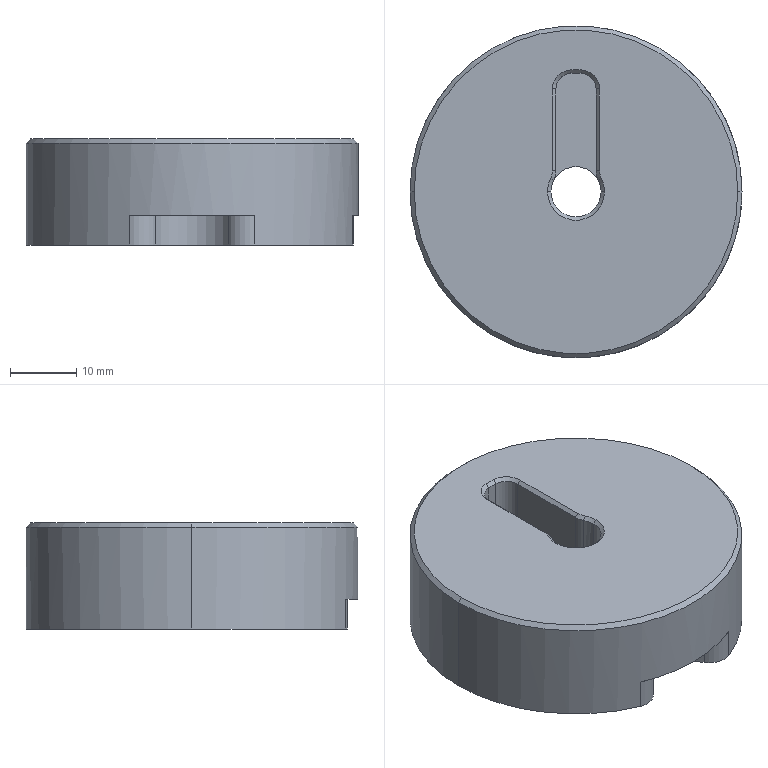Part | 1 solid | 47 faces | box 50.292 x 50.292 x 16.057 mm | volume 28762 mm3 | cylinder 23 | plane 14 | cone 10 | commonest cylinder face diameters 6.35 x8 4.763 x5 5.067 x4 7.62 x2 50.292 x2 12.7 x1
STEP:
#1=CARTESIAN_POINT('',(24.432,-5.556,-16.057));
#2=VERTEX_POINT('',#1);
#3=CARTESIAN_POINT('',(24.329,-6.359,-16.057));
#4=VERTEX_POINT('',#3);
#5=CARTESIAN_POINT('',(21.257,-5.556,-16.057));
#6=DIRECTION('',(0.,0.,-1.));
#7=DIRECTION('',(-1.,0.,0.));
#8=AXIS2_PLACEMENT_3D('',#5,#6,#7);
#9=CIRCLE('',#8,3.175);
#10=EDGE_CURVE('',#2,#4,#9,.T.);
#11=ORIENTED_EDGE('',*,*,#10,.F.);
#12=CARTESIAN_POINT('',(24.432,-5.556,-11.579));
#13=VERTEX_POINT('',#12);
#14=CARTESIAN_POINT('',(24.432,-5.556,0.));
#15=DIRECTION('',(0.,0.,-1.));
#16=VECTOR('',#15,1000.);
#17=LINE('',#14,#16);
#18=EDGE_CURVE('',#13,#2,#17,.T.);
#19=ORIENTED_EDGE('',*,*,#18,.F.);
#20=CARTESIAN_POINT('',(24.329,-6.359,-11.579));
#21=VERTEX_POINT('',#20);
#22=CARTESIAN_POINT('',(21.257,-5.556,-11.579));
#23=DIRECTION('',(0.,0.,1.));
#24=DIRECTION('',(1.,0.,0.));
#25=AXIS2_PLACEMENT_3D('',#22,#23,#24);
#26=CIRCLE('',#25,3.175);
#27=EDGE_CURVE('',#21,#13,#26,.T.);
#28=ORIENTED_EDGE('',*,*,#27,.F.);
#29=CARTESIAN_POINT('',(24.329,-6.359,0.));
#30=DIRECTION('',(0.,0.,1.));
#31=VECTOR('',#30,1000.);
#32=LINE('',#29,#31);
#33=EDGE_CURVE('',#4,#21,#32,.T.);
#34=ORIENTED_EDGE('',*,*,#33,.F.);
#35=EDGE_LOOP('',(#11,#19,#28,#34));
#36=FACE_BOUND('',#35,.T.);
#37=CARTESIAN_POINT('',(21.257,-5.556,0.));
#38=DIRECTION('',(0.,0.,-1.));
#39=DIRECTION('',(-1.,0.,0.));
#40=AXIS2_PLACEMENT_3D('',#37,#38,#39);
#41=CYLINDRICAL_SURFACE('',#40,3.175);
#42=ADVANCED_FACE('',(#36),#41,.T.);
#43=CARTESIAN_POINT('',(21.257,-2.381,-16.057));
#44=VERTEX_POINT('',#43);
#45=CARTESIAN_POINT('',(21.257,-5.556,-16.057));
#46=DIRECTION('',(0.,0.,-1.));
#47=DIRECTION('',(-1.,0.,0.));
#48=AXIS2_PLACEMENT_3D('',#45,#46,#47);
#49=CIRCLE('',#48,3.175);
#50=EDGE_CURVE('',#44,#2,#49,.T.);
#51=ORIENTED_EDGE('',*,*,#50,.F.);
#52=CARTESIAN_POINT('',(21.257,-2.381,-11.579));
#53=VERTEX_POINT('',#52);
#54=CARTESIAN_POINT('',(21.257,-2.381,-11.579));
#55=DIRECTION('',(0.,0.,-1.));
#56=VECTOR('',#55,1000.);
#57=LINE('',#54,#56);
#58=EDGE_CURVE('',#53,#44,#57,.T.);
#59=ORIENTED_EDGE('',*,*,#58,.F.);
#60=CARTESIAN_POINT('',(21.257,-5.556,-11.579));
#61=DIRECTION('',(0.,0.,1.));
#62=DIRECTION('',(1.,0.,0.));
#63=AXIS2_PLACEMENT_3D('',#60,#61,#62);
#64=CIRCLE('',#63,3.175);
#65=EDGE_CURVE('',#13,#53,#64,.T.);
#66=ORIENTED_EDGE('',*,*,#65,.F.);
#67=ORIENTED_EDGE('',*,*,#18,.T.);
#68=EDGE_LOOP('',(#51,#59,#66,#67));
#69=FACE_BOUND('',#68,.T.);
#70=CARTESIAN_POINT('',(21.257,-5.556,0.));
#71=DIRECTION('',(0.,0.,-1.));
#72=DIRECTION('',(-1.,0.,0.));
#73=AXIS2_PLACEMENT_3D('',#70,#71,#72);
#74=CYLINDRICAL_SURFACE('',#73,3.175);
#75=ADVANCED_FACE('',(#69),#74,.T.);
#76=ORIENTED_EDGE('',*,*,#58,.T.);
#77=CARTESIAN_POINT('',(12.898,-2.381,-16.057));
#78=VERTEX_POINT('',#77);
#79=CARTESIAN_POINT('',(12.898,-2.381,-16.057));
#80=DIRECTION('',(-1.,0.,0.));
#81=VECTOR('',#80,1000.);
#82=LINE('',#79,#81);
#83=EDGE_CURVE('',#44,#78,#82,.T.);
#84=ORIENTED_EDGE('',*,*,#83,.T.);
#85=CARTESIAN_POINT('',(12.898,-2.381,-11.579));
#86=VERTEX_POINT('',#85);
#87=CARTESIAN_POINT('',(12.898,-2.381,-11.579));
#88=DIRECTION('',(0.,0.,-1.));
#89=VECTOR('',#88,1000.);
#90=LINE('',#87,#89);
#91=EDGE_CURVE('',#86,#78,#90,.T.);
#92=ORIENTED_EDGE('',*,*,#91,.F.);
#93=CARTESIAN_POINT('',(12.898,-2.381,-11.579));
#94=DIRECTION('',(-1.,0.,0.));
#95=VECTOR('',#94,1000.);
#96=LINE('',#93,#95);
#97=EDGE_CURVE('',#53,#86,#96,.T.);
#98=ORIENTED_EDGE('',*,*,#97,.F.);
#99=EDGE_LOOP('',(#76,#84,#92,#98));
#100=FACE_BOUND('',#99,.T.);
#101=CARTESIAN_POINT('',(12.898,-2.381,-11.579));
#102=DIRECTION('',(0.,-1.,0.));
#103=DIRECTION('',(1.,0.,0.));
#104=AXIS2_PLACEMENT_3D('',#101,#102,#103);
#105=PLANE('',#104);
#106=ADVANCED_FACE('',(#100),#105,.F.);
#107=ORIENTED_EDGE('',*,*,#91,.T.);
#108=CARTESIAN_POINT('',(11.168,1.636,-16.057));
#109=VERTEX_POINT('',#108);
#110=CARTESIAN_POINT('',(12.898,0.,-16.057));
#111=DIRECTION('',(0.,0.,-1.));
#112=DIRECTION('',(-1.,0.,0.));
#113=AXIS2_PLACEMENT_3D('',#110,#111,#112);
#114=CIRCLE('',#113,2.381);
#115=EDGE_CURVE('',#78,#109,#114,.T.);
#116=ORIENTED_EDGE('',*,*,#115,.T.);
#117=CARTESIAN_POINT('',(11.168,1.636,-11.579));
#118=VERTEX_POINT('',#117);
#119=CARTESIAN_POINT('',(11.168,1.636,-11.579));
#120=DIRECTION('',(0.,0.,-1.));
#121=VECTOR('',#120,1000.);
#122=LINE('',#119,#121);
#123=EDGE_CURVE('',#118,#109,#122,.T.);
#124=ORIENTED_EDGE('',*,*,#123,.F.);
#125=CARTESIAN_POINT('',(12.898,0.,-11.579));
#126=DIRECTION('',(0.,0.,-1.));
#127=DIRECTION('',(1.,0.,0.));
#128=AXIS2_PLACEMENT_3D('',#125,#126,#127);
#129=CIRCLE('',#128,2.381);
#130=EDGE_CURVE('',#86,#118,#129,.T.);
#131=ORIENTED_EDGE('',*,*,#130,.F.);
#132=EDGE_LOOP('',(#107,#116,#124,#131));
#133=FACE_BOUND('',#132,.T.);
#134=CARTESIAN_POINT('',(12.898,0.,-11.579));
#135=DIRECTION('',(0.,0.,-1.));
#136=DIRECTION('',(-1.,0.,0.));
#137=AXIS2_PLACEMENT_3D('',#134,#135,#136);
#138=CYLINDRICAL_SURFACE('',#137,2.381);
#139=ADVANCED_FACE('',(#133),#138,.F.);
#140=ORIENTED_EDGE('',*,*,#123,.T.);
#141=CARTESIAN_POINT('',(19.946,10.918,-16.057));
#142=VERTEX_POINT('',#141);
#143=CARTESIAN_POINT('',(16.338,7.102,-16.057));
#144=DIRECTION('',(0.6871,0.7266,0.));
#145=VECTOR('',#144,1000.);
#146=LINE('',#143,#145);
#147=EDGE_CURVE('',#109,#142,#146,.T.);
#148=ORIENTED_EDGE('',*,*,#147,.T.);
#149=CARTESIAN_POINT('',(19.946,10.918,-11.579));
#150=VERTEX_POINT('',#149);
#151=CARTESIAN_POINT('',(19.946,10.918,-11.579));
#152=DIRECTION('',(0.,0.,1.));
#153=VECTOR('',#152,1000.);
#154=LINE('',#151,#153);
#155=EDGE_CURVE('',#142,#150,#154,.T.);
#156=ORIENTED_EDGE('',*,*,#155,.T.);
#157=CARTESIAN_POINT('',(16.338,7.102,-11.579));
#158=DIRECTION('',(0.6871,0.7266,0.));
#159=VECTOR('',#158,1000.);
#160=LINE('',#157,#159);
#161=EDGE_CURVE('',#118,#150,#160,.T.);
#162=ORIENTED_EDGE('',*,*,#161,.F.);
#163=EDGE_LOOP('',(#140,#148,#156,#162));
#164=FACE_BOUND('',#163,.T.);
#165=CARTESIAN_POINT('',(16.338,7.102,-11.579));
#166=DIRECTION('',(-0.7266,0.6871,0.));
#167=DIRECTION('',(0.,0.,1.));
#168=AXIS2_PLACEMENT_3D('',#165,#166,#167);
#169=PLANE('',#168);
#170=ADVANCED_FACE('',(#164),#169,.F.);
#171=CARTESIAN_POINT('',(20.814,13.099,-16.057));
#172=VERTEX_POINT('',#171);
#173=CARTESIAN_POINT('',(17.639,13.099,-16.057));
#174=DIRECTION('',(0.,0.,-1.));
#175=DIRECTION('',(-1.,0.,0.));
#176=AXIS2_PLACEMENT_3D('',#173,#174,#175);
#177=CIRCLE('',#176,3.175);
#178=EDGE_CURVE('',#172,#142,#177,.T.);
#179=ORIENTED_EDGE('',*,*,#178,.F.);
#180=CARTESIAN_POINT('',(20.814,13.099,-11.579));
#181=VERTEX_POINT('',#180);
#182=CARTESIAN_POINT('',(20.814,13.099,0.));
#183=DIRECTION('',(0.,0.,-1.));
#184=VECTOR('',#183,1000.);
#185=LINE('',#182,#184);
#186=EDGE_CURVE('',#181,#172,#185,.T.);
#187=ORIENTED_EDGE('',*,*,#186,.F.);
#188=CARTESIAN_POINT('',(17.639,13.099,-11.579));
#189=DIRECTION('',(0.,0.,1.));
#190=DIRECTION('',(1.,0.,0.));
#191=AXIS2_PLACEMENT_3D('',#188,#189,#190);
#192=CIRCLE('',#191,3.175);
#193=EDGE_CURVE('',#150,#181,#192,.T.);
#194=ORIENTED_EDGE('',*,*,#193,.F.);
#195=ORIENTED_EDGE('',*,*,#155,.F.);
#196=EDGE_LOOP('',(#179,#187,#194,#195));
#197=FACE_BOUND('',#196,.T.);
#198=CARTESIAN_POINT('',(17.639,13.099,0.));
#199=DIRECTION('',(0.,0.,-1.));
#200=DIRECTION('',(-1.,0.,0.));
#201=AXIS2_PLACEMENT_3D('',#198,#199,#200);
#202=CYLINDRICAL_SURFACE('',#201,3.175);
#203=ADVANCED_FACE('',(#197),#202,.T.);
#204=CARTESIAN_POINT('',(20.188,14.992,-16.057));
#205=VERTEX_POINT('',#204);
#206=CARTESIAN_POINT('',(17.639,13.099,-16.057));
#207=DIRECTION('',(0.,0.,-1.));
#208=DIRECTION('',(-1.,0.,0.));
#209=AXIS2_PLACEMENT_3D('',#206,#207,#208);
#210=CIRCLE('',#209,3.175);
#211=EDGE_CURVE('',#205,#172,#210,.T.);
#212=ORIENTED_EDGE('',*,*,#211,.F.);
#213=CARTESIAN_POINT('',(20.188,14.992,-11.579));
#214=VERTEX_POINT('',#213);
#215=CARTESIAN_POINT('',(20.188,14.992,0.));
#216=DIRECTION('',(0.,0.,-1.));
#217=VECTOR('',#216,1000.);
#218=LINE('',#215,#217);
#219=EDGE_CURVE('',#214,#205,#218,.T.);
#220=ORIENTED_EDGE('',*,*,#219,.F.);
#221=CARTESIAN_POINT('',(17.639,13.099,-11.579));
#222=DIRECTION('',(0.,0.,1.));
#223=DIRECTION('',(1.,0.,0.));
#224=AXIS2_PLACEMENT_3D('',#221,#222,#223);
#225=CIRCLE('',#224,3.175);
#226=EDGE_CURVE('',#181,#214,#225,.T.);
#227=ORIENTED_EDGE('',*,*,#226,.F.);
#228=ORIENTED_EDGE('',*,*,#186,.T.);
#229=EDGE_LOOP('',(#212,#220,#227,#228));
#230=FACE_BOUND('',#229,.T.);
#231=CARTESIAN_POINT('',(17.639,13.099,0.));
#232=DIRECTION('',(0.,0.,-1.));
#233=DIRECTION('',(-1.,0.,0.));
#234=AXIS2_PLACEMENT_3D('',#231,#232,#233);
#235=CYLINDRICAL_SURFACE('',#234,3.175);
#236=ADVANCED_FACE('',(#230),#235,.T.);
#237=CARTESIAN_POINT('',(-25.146,0.,-16.057));
#238=VERTEX_POINT('',#237);
#239=CARTESIAN_POINT('',(0.,0.,-16.057));
#240=DIRECTION('',(0.,0.,-1.));
#241=DIRECTION('',(-1.,0.,0.));
#242=AXIS2_PLACEMENT_3D('',#239,#240,#241);
#243=CIRCLE('',#242,25.146);
#244=EDGE_CURVE('',#238,#205,#243,.T.);
#245=ORIENTED_EDGE('',*,*,#244,.F.);
#246=CARTESIAN_POINT('',(-25.146,0.,-0.635));
#247=VERTEX_POINT('',#246);
#248=CARTESIAN_POINT('',(-25.146,0.,0.));
#249=DIRECTION('',(0.,0.,-1.));
#250=VECTOR('',#249,1000.);
#251=LINE('',#248,#250);
#252=EDGE_CURVE('',#238,#247,#251,.F.);
#253=ORIENTED_EDGE('',*,*,#252,.T.);
#254=CARTESIAN_POINT('',(25.146,0.,-0.635));
#255=VERTEX_POINT('',#254);
#256=CARTESIAN_POINT('',(0.,0.,-0.635));
#257=DIRECTION('',(0.,0.,-1.));
#258=DIRECTION('',(-1.,0.,0.));
#259=AXIS2_PLACEMENT_3D('',#256,#257,#258);
#260=CIRCLE('',#259,25.146);
#261=EDGE_CURVE('',#247,#255,#260,.T.);
#262=ORIENTED_EDGE('',*,*,#261,.T.);
#263=CARTESIAN_POINT('',(25.146,0.,-11.579));
#264=VERTEX_POINT('',#263);
#265=CARTESIAN_POINT('',(25.146,0.,0.));
#266=DIRECTION('',(0.,0.,-1.));
#267=VECTOR('',#266,1000.);
#268=LINE('',#265,#267);
#269=EDGE_CURVE('',#264,#255,#268,.F.);
#270=ORIENTED_EDGE('',*,*,#269,.F.);
#271=CARTESIAN_POINT('',(0.,0.,-11.579));
#272=DIRECTION('',(0.,0.,-1.));
#273=DIRECTION('',(1.,0.,0.));
#274=AXIS2_PLACEMENT_3D('',#271,#272,#273);
#275=CIRCLE('',#274,25.146);
#276=EDGE_CURVE('',#214,#264,#275,.T.);
#277=ORIENTED_EDGE('',*,*,#276,.F.);
#278=ORIENTED_EDGE('',*,*,#219,.T.);
#279=EDGE_LOOP('',(#245,#253,#262,#270,#277,#278));
#280=FACE_BOUND('',#279,.T.);
#281=CARTESIAN_POINT('',(0.,0.,0.));
#282=DIRECTION('',(0.,0.,-1.));
#283=DIRECTION('',(-1.,0.,0.));
#284=AXIS2_PLACEMENT_3D('',#281,#282,#283);
#285=CYLINDRICAL_SURFACE('',#284,25.146);
#286=ADVANCED_FACE('',(#280),#285,.T.);
#287=CARTESIAN_POINT('',(9.464,-23.297,-16.057));
#288=VERTEX_POINT('',#287);
#289=CARTESIAN_POINT('',(0.,0.,-16.057));
#290=DIRECTION('',(0.,0.,-1.));
#291=DIRECTION('',(-1.,0.,0.));
#292=AXIS2_PLACEMENT_3D('',#289,#290,#291);
#293=CIRCLE('',#292,25.146);
#294=EDGE_CURVE('',#4,#288,#293,.T.);
#295=ORIENTED_EDGE('',*,*,#294,.F.);
#296=ORIENTED_EDGE('',*,*,#33,.T.);
#297=CARTESIAN_POINT('',(0.,0.,-11.579));
#298=DIRECTION('',(0.,0.,-1.));
#299=DIRECTION('',(1.,0.,0.));
#300=AXIS2_PLACEMENT_3D('',#297,#298,#299);
#301=CIRCLE('',#300,25.146);
#302=EDGE_CURVE('',#264,#21,#301,.T.);
#303=ORIENTED_EDGE('',*,*,#302,.F.);
#304=ORIENTED_EDGE('',*,*,#269,.T.);
#305=CARTESIAN_POINT('',(0.,0.,-0.635));
#306=DIRECTION('',(0.,0.,-1.));
#307=DIRECTION('',(-1.,0.,0.));
#308=AXIS2_PLACEMENT_3D('',#305,#306,#307);
#309=CIRCLE('',#308,25.146);
#310=EDGE_CURVE('',#255,#247,#309,.T.);
#311=ORIENTED_EDGE('',*,*,#310,.T.);
#312=ORIENTED_EDGE('',*,*,#252,.F.);
#313=CARTESIAN_POINT('',(-9.464,-23.297,-16.057));
#314=VERTEX_POINT('',#313);
#315=CARTESIAN_POINT('',(0.,0.,-16.057));
#316=DIRECTION('',(0.,0.,-1.));
#317=DIRECTION('',(-1.,0.,0.));
#318=AXIS2_PLACEMENT_3D('',#315,#316,#317);
#319=CIRCLE('',#318,25.146);
#320=EDGE_CURVE('',#314,#238,#319,.T.);
#321=ORIENTED_EDGE('',*,*,#320,.F.);
#322=CARTESIAN_POINT('',(-9.464,-23.297,-11.579));
#323=VERTEX_POINT('',#322);
#324=CARTESIAN_POINT('',(-9.464,-23.297,0.));
#325=DIRECTION('',(0.,0.,1.));
#326=VECTOR('',#325,1000.);
#327=LINE('',#324,#326);
#328=EDGE_CURVE('',#314,#323,#327,.T.);
#329=ORIENTED_EDGE('',*,*,#328,.T.);
#330=CARTESIAN_POINT('',(9.464,-23.297,-11.579));
#331=VERTEX_POINT('',#330);
#332=CARTESIAN_POINT('',(0.,0.,-11.579));
#333=DIRECTION('',(0.,0.,-1.));
#334=DIRECTION('',(1.,0.,0.));
#335=AXIS2_PLACEMENT_3D('',#332,#333,#334);
#336=CIRCLE('',#335,25.146);
#337=EDGE_CURVE('',#331,#323,#336,.T.);
#338=ORIENTED_EDGE('',*,*,#337,.F.);
#339=CARTESIAN_POINT('',(9.464,-23.297,0.));
#340=DIRECTION('',(0.,0.,-1.));
#341=VECTOR('',#340,1000.);
#342=LINE('',#339,#341);
#343=EDGE_CURVE('',#331,#288,#342,.T.);
#344=ORIENTED_EDGE('',*,*,#343,.T.);
#345=EDGE_LOOP('',(#295,#296,#303,#304,#311,#312,#321,#329,#338,#344));
#346=FACE_BOUND('',#345,.T.);
#347=CARTESIAN_POINT('',(0.,0.,0.));
#348=DIRECTION('',(0.,0.,-1.));
#349=DIRECTION('',(-1.,0.,0.));
#350=AXIS2_PLACEMENT_3D('',#347,#348,#349);
#351=CYLINDRICAL_SURFACE('',#350,25.146);
#352=ADVANCED_FACE('',(#346),#351,.T.);
#353=CARTESIAN_POINT('',(-3.048,15.574,-0.508));
#354=VERTEX_POINT('',#353);
#355=CARTESIAN_POINT('',(-3.556,15.574,0.));
#356=VERTEX_POINT('',#355);
#357=CARTESIAN_POINT('',(-3.048,15.574,-0.508));
#358=DIRECTION('',(-0.7071,0.,0.7071));
#359=VECTOR('',#358,1000.);
#360=LINE('',#357,#359);
#361=EDGE_CURVE('',#354,#356,#360,.T.);
#362=ORIENTED_EDGE('',*,*,#361,.T.);
#363=CARTESIAN_POINT('',(-3.556,3.172,0.));
#364=VERTEX_POINT('',#363);
#365=CARTESIAN_POINT('',(-3.556,0.,0.));
#366=DIRECTION('',(0.,1.,0.));
#367=VECTOR('',#366,1000.);
#368=LINE('',#365,#367);
#369=EDGE_CURVE('',#364,#356,#368,.T.);
#370=ORIENTED_EDGE('',*,*,#369,.F.);
#371=CARTESIAN_POINT('',(-3.048,3.172,-0.508));
#372=VERTEX_POINT('',#371);
#373=CARTESIAN_POINT('',(-3.556,3.172,0.));
#374=DIRECTION('',(0.7071,0.,-0.7071));
#375=VECTOR('',#374,1000.);
#376=LINE('',#373,#375);
#377=EDGE_CURVE('',#364,#372,#376,.T.);
#378=ORIENTED_EDGE('',*,*,#377,.T.);
#379=CARTESIAN_POINT('',(-3.048,0.,-0.508));
#380=DIRECTION('',(0.,-1.,0.));
#381=VECTOR('',#380,1000.);
#382=LINE('',#379,#381);
#383=EDGE_CURVE('',#354,#372,#382,.T.);
#384=ORIENTED_EDGE('',*,*,#383,.F.);
#385=EDGE_LOOP('',(#362,#370,#378,#384));
#386=FACE_BOUND('',#385,.T.);
#387=CARTESIAN_POINT('',(-3.048,0.,-0.508));
#388=DIRECTION('',(-0.7071,0.,-0.7071));
#389=DIRECTION('',(0.,-1.,0.));
#390=AXIS2_PLACEMENT_3D('',#387,#388,#389);
#391=PLANE('',#390);
#392=ADVANCED_FACE('',(#386),#391,.F.);
#393=CARTESIAN_POINT('',(-3.847,1.961,0.));
#394=VERTEX_POINT('',#393);
#395=CARTESIAN_POINT('',(-3.394,1.73,-0.508));
#396=VERTEX_POINT('',#395);
#397=CARTESIAN_POINT('',(-3.847,1.961,0.));
#398=DIRECTION('',(0.63,-0.3212,-0.7071));
#399=VECTOR('',#398,1000.);
#400=LINE('',#397,#399);
#401=EDGE_CURVE('',#394,#396,#400,.T.);
#402=ORIENTED_EDGE('',*,*,#401,.T.);
#403=CARTESIAN_POINT('',(-6.223,3.172,-0.508));
#404=DIRECTION('',(0.,0.,-1.));
#405=DIRECTION('',(-1.,0.,0.));
#406=AXIS2_PLACEMENT_3D('',#403,#404,#405);
#407=CIRCLE('',#406,3.175);
#408=EDGE_CURVE('',#372,#396,#407,.T.);
#409=ORIENTED_EDGE('',*,*,#408,.F.);
#410=ORIENTED_EDGE('',*,*,#377,.F.);
#411=CARTESIAN_POINT('',(-6.223,3.172,0.));
#412=DIRECTION('',(0.,0.,1.));
#413=DIRECTION('',(-1.,0.,0.));
#414=AXIS2_PLACEMENT_3D('',#411,#412,#413);
#415=CIRCLE('',#414,2.667);
#416=EDGE_CURVE('',#394,#364,#415,.T.);
#417=ORIENTED_EDGE('',*,*,#416,.F.);
#418=EDGE_LOOP('',(#402,#409,#410,#417));
#419=FACE_BOUND('',#418,.T.);
#420=CARTESIAN_POINT('',(-6.223,3.172,0.));
#421=DIRECTION('',(0.,0.,-1.));
#422=DIRECTION('',(-1.,0.,0.));
#423=AXIS2_PLACEMENT_3D('',#420,#421,#422);
#424=CONICAL_SURFACE('',#423,2.667,0.7854);
#425=ADVANCED_FACE('',(#419),#424,.T.);
#426=CARTESIAN_POINT('',(-0.7776,17.952,-0.508));
#427=VERTEX_POINT('',#426);
#428=CARTESIAN_POINT('',(-0.8013,18.46,0.));
#429=VERTEX_POINT('',#428);
#430=CARTESIAN_POINT('',(-0.7776,17.952,-0.508));
#431=DIRECTION('',(-0.03293,0.7063,0.7071));
#432=VECTOR('',#431,1000.);
#433=LINE('',#430,#432);
#434=EDGE_CURVE('',#427,#429,#433,.T.);
#435=ORIENTED_EDGE('',*,*,#434,.T.);
#436=CARTESIAN_POINT('',(-0.6667,15.574,0.));
#437=DIRECTION('',(0.,0.,-1.));
#438=DIRECTION('',(-1.,0.,0.));
#439=AXIS2_PLACEMENT_3D('',#436,#437,#438);
#440=CIRCLE('',#439,2.889);
#441=EDGE_CURVE('',#356,#429,#440,.T.);
#442=ORIENTED_EDGE('',*,*,#441,.F.);
#443=ORIENTED_EDGE('',*,*,#361,.F.);
#444=CARTESIAN_POINT('',(-0.6667,15.574,-0.508));
#445=DIRECTION('',(0.,0.,1.));
#446=DIRECTION('',(-1.,0.,0.));
#447=AXIS2_PLACEMENT_3D('',#444,#445,#446);
#448=CIRCLE('',#447,2.381);
#449=EDGE_CURVE('',#427,#354,#448,.T.);
#450=ORIENTED_EDGE('',*,*,#449,.F.);
#451=EDGE_LOOP('',(#435,#442,#443,#450));
#452=FACE_BOUND('',#451,.T.);
#453=CARTESIAN_POINT('',(-0.6667,15.574,0.));
#454=DIRECTION('',(0.,0.,1.));
#455=DIRECTION('',(1.,0.,0.));
#456=AXIS2_PLACEMENT_3D('',#453,#454,#455);
#457=CONICAL_SURFACE('',#456,2.889,0.7854);
#458=ADVANCED_FACE('',(#452),#457,.F.);
#459=CARTESIAN_POINT('',(-3.81,0.,-0.508));
#460=VERTEX_POINT('',#459);
#461=CARTESIAN_POINT('',(-4.318,0.,0.));
#462=VERTEX_POINT('',#461);
#463=CARTESIAN_POINT('',(-3.81,0.,-0.508));
#464=DIRECTION('',(-0.7071,0.,0.7071));
#465=VECTOR('',#464,1000.);
#466=LINE('',#463,#465);
#467=EDGE_CURVE('',#460,#462,#466,.T.);
#468=ORIENTED_EDGE('',*,*,#467,.F.);
#469=CARTESIAN_POINT('',(0.,0.,-0.508));
#470=DIRECTION('',(0.,0.,1.));
#471=DIRECTION('',(-1.,0.,0.));
#472=AXIS2_PLACEMENT_3D('',#469,#470,#471);
#473=CIRCLE('',#472,3.81);
#474=EDGE_CURVE('',#396,#460,#473,.T.);
#475=ORIENTED_EDGE('',*,*,#474,.F.);
#476=ORIENTED_EDGE('',*,*,#401,.F.);
#477=CARTESIAN_POINT('',(0.,0.,0.));
#478=DIRECTION('',(0.,0.,-1.));
#479=DIRECTION('',(-1.,0.,0.));
#480=AXIS2_PLACEMENT_3D('',#477,#478,#479);
#481=CIRCLE('',#480,4.318);
#482=EDGE_CURVE('',#462,#394,#481,.T.);
#483=ORIENTED_EDGE('',*,*,#482,.F.);
#484=EDGE_LOOP('',(#468,#475,#476,#483));
#485=FACE_BOUND('',#484,.T.);
#486=CARTESIAN_POINT('',(0.,0.,-0.508));
#487=DIRECTION('',(0.,0.,1.));
#488=DIRECTION('',(1.,0.,0.));
#489=AXIS2_PLACEMENT_3D('',#486,#487,#488);
#490=CONICAL_SURFACE('',#489,3.81,0.7854);
#491=ADVANCED_FACE('',(#485),#490,.F.);
#492=CARTESIAN_POINT('',(0.7776,17.952,-0.508));
#493=VERTEX_POINT('',#492);
#494=CARTESIAN_POINT('',(0.8013,18.46,0.));
#495=VERTEX_POINT('',#494);
#496=CARTESIAN_POINT('',(0.7776,17.952,-0.508));
#497=DIRECTION('',(0.03293,0.7063,0.7071));
#498=VECTOR('',#497,1000.);
#499=LINE('',#496,#498);
#500=EDGE_CURVE('',#493,#495,#499,.T.);
#501=ORIENTED_EDGE('',*,*,#500,.T.);
#502=CARTESIAN_POINT('',(0.,1.27,0.));
#503=DIRECTION('',(0.,0.,-1.));
#504=DIRECTION('',(-1.,0.,0.));
#505=AXIS2_PLACEMENT_3D('',#502,#503,#504);
#506=CIRCLE('',#505,17.209);
#507=EDGE_CURVE('',#429,#495,#506,.T.);
#508=ORIENTED_EDGE('',*,*,#507,.F.);
#509=ORIENTED_EDGE('',*,*,#434,.F.);
#510=CARTESIAN_POINT('',(0.,1.27,-0.508));
#511=DIRECTION('',(0.,0.,1.));
#512=DIRECTION('',(-1.,0.,0.));
#513=AXIS2_PLACEMENT_3D('',#510,#511,#512);
#514=CIRCLE('',#513,16.701);
#515=EDGE_CURVE('',#493,#427,#514,.T.);
#516=ORIENTED_EDGE('',*,*,#515,.F.);
#517=EDGE_LOOP('',(#501,#508,#509,#516));
#518=FACE_BOUND('',#517,.T.);
#519=CARTESIAN_POINT('',(0.,1.27,-0.508));
#520=DIRECTION('',(0.,0.,1.));
#521=DIRECTION('',(1.,0.,0.));
#522=AXIS2_PLACEMENT_3D('',#519,#520,#521);
#523=CONICAL_SURFACE('',#522,16.701,0.7854);
#524=ADVANCED_FACE('',(#518),#523,.F.);
#525=CARTESIAN_POINT('',(3.556,3.172,0.));
#526=VERTEX_POINT('',#525);
#527=CARTESIAN_POINT('',(3.048,3.172,-0.508));
#528=VERTEX_POINT('',#527);
#529=CARTESIAN_POINT('',(3.556,3.172,0.));
#530=DIRECTION('',(-0.7071,0.,-0.7071));
#531=VECTOR('',#530,1000.);
#532=LINE('',#529,#531);
#533=EDGE_CURVE('',#526,#528,#532,.T.);
#534=ORIENTED_EDGE('',*,*,#533,.T.);
#535=CARTESIAN_POINT('',(3.394,1.73,-0.508));
#536=VERTEX_POINT('',#535);
#537=CARTESIAN_POINT('',(6.223,3.172,-0.508));
#538=DIRECTION('',(0.,0.,-1.));
#539=DIRECTION('',(-1.,0.,0.));
#540=AXIS2_PLACEMENT_3D('',#537,#538,#539);
#541=CIRCLE('',#540,3.175);
#542=EDGE_CURVE('',#536,#528,#541,.T.);
#543=ORIENTED_EDGE('',*,*,#542,.F.);
#544=CARTESIAN_POINT('',(3.847,1.961,0.));
#545=VERTEX_POINT('',#544);
#546=CARTESIAN_POINT('',(3.847,1.961,0.));
#547=DIRECTION('',(-0.63,-0.3212,-0.7071));
#548=VECTOR('',#547,1000.);
#549=LINE('',#546,#548);
#550=EDGE_CURVE('',#545,#536,#549,.T.);
#551=ORIENTED_EDGE('',*,*,#550,.F.);
#552=CARTESIAN_POINT('',(6.223,3.172,0.));
#553=DIRECTION('',(0.,0.,1.));
#554=DIRECTION('',(-1.,0.,0.));
#555=AXIS2_PLACEMENT_3D('',#552,#553,#554);
#556=CIRCLE('',#555,2.667);
#557=EDGE_CURVE('',#526,#545,#556,.T.);
#558=ORIENTED_EDGE('',*,*,#557,.F.);
#559=EDGE_LOOP('',(#534,#543,#551,#558));
#560=FACE_BOUND('',#559,.T.);
#561=CARTESIAN_POINT('',(6.223,3.172,0.));
#562=DIRECTION('',(0.,0.,-1.));
#563=DIRECTION('',(-1.,0.,0.));
#564=AXIS2_PLACEMENT_3D('',#561,#562,#563);
#565=CONICAL_SURFACE('',#564,2.667,0.7854);
#566=ADVANCED_FACE('',(#560),#565,.T.);
#567=CARTESIAN_POINT('',(3.048,15.574,-0.508));
#568=VERTEX_POINT('',#567);
#569=CARTESIAN_POINT('',(3.556,15.574,0.));
#570=VERTEX_POINT('',#569);
#571=CARTESIAN_POINT('',(3.048,15.574,-0.508));
#572=DIRECTION('',(0.7071,0.,0.7071));
#573=VECTOR('',#572,1000.);
#574=LINE('',#571,#573);
#575=EDGE_CURVE('',#568,#570,#574,.T.);
#576=ORIENTED_EDGE('',*,*,#575,.T.);
#577=CARTESIAN_POINT('',(0.6667,15.574,0.));
#578=DIRECTION('',(0.,0.,-1.));
#579=DIRECTION('',(-1.,0.,0.));
#580=AXIS2_PLACEMENT_3D('',#577,#578,#579);
#581=CIRCLE('',#580,2.889);
#582=EDGE_CURVE('',#495,#570,#581,.T.);
#583=ORIENTED_EDGE('',*,*,#582,.F.);
#584=ORIENTED_EDGE('',*,*,#500,.F.);
#585=CARTESIAN_POINT('',(0.6667,15.574,-0.508));
#586=DIRECTION('',(0.,0.,1.));
#587=DIRECTION('',(-1.,0.,0.));
#588=AXIS2_PLACEMENT_3D('',#585,#586,#587);
#589=CIRCLE('',#588,2.381);
#590=EDGE_CURVE('',#568,#493,#589,.T.);
#591=ORIENTED_EDGE('',*,*,#590,.F.);
#592=EDGE_LOOP('',(#576,#583,#584,#591));
#593=FACE_BOUND('',#592,.T.);
#594=CARTESIAN_POINT('',(0.6667,15.574,0.));
#595=DIRECTION('',(0.,0.,1.));
#596=DIRECTION('',(1.,0.,0.));
#597=AXIS2_PLACEMENT_3D('',#594,#595,#596);
#598=CONICAL_SURFACE('',#597,2.889,0.7854);
#599=ADVANCED_FACE('',(#593),#598,.F.);
#600=ORIENTED_EDGE('',*,*,#533,.F.);
#601=CARTESIAN_POINT('',(3.556,0.,0.));
#602=DIRECTION('',(0.,-1.,0.));
#603=VECTOR('',#602,1000.);
#604=LINE('',#601,#603);
#605=EDGE_CURVE('',#570,#526,#604,.T.);
#606=ORIENTED_EDGE('',*,*,#605,.F.);
#607=ORIENTED_EDGE('',*,*,#575,.F.);
#608=CARTESIAN_POINT('',(3.048,0.,-0.508));
#609=DIRECTION('',(0.,1.,0.));
#610=VECTOR('',#609,1000.);
#611=LINE('',#608,#610);
#612=EDGE_CURVE('',#528,#568,#611,.T.);
#613=ORIENTED_EDGE('',*,*,#612,.F.);
#614=EDGE_LOOP('',(#600,#606,#607,#613));
#615=FACE_BOUND('',#614,.T.);
#616=CARTESIAN_POINT('',(3.048,0.,-0.508));
#617=DIRECTION('',(0.7071,0.,-0.7071));
#618=DIRECTION('',(-0.7071,0.,-0.7071));
#619=AXIS2_PLACEMENT_3D('',#616,#617,#618);
#620=PLANE('',#619);
#621=ADVANCED_FACE('',(#615),#620,.F.);
#622=CARTESIAN_POINT('',(-24.511,0.,0.));
#623=VERTEX_POINT('',#622);
#624=CARTESIAN_POINT('',(-24.511,0.,0.));
#625=DIRECTION('',(-0.7071,0.,-0.7071));
#626=VECTOR('',#625,1000.);
#627=LINE('',#624,#626);
#628=EDGE_CURVE('',#247,#623,#627,.F.);
#629=ORIENTED_EDGE('',*,*,#628,.T.);
#630=CARTESIAN_POINT('',(24.511,0.,0.));
#631=VERTEX_POINT('',#630);
#632=CARTESIAN_POINT('',(0.,0.,0.));
#633=DIRECTION('',(0.,0.,1.));
#634=DIRECTION('',(-1.,0.,0.));
#635=AXIS2_PLACEMENT_3D('',#632,#633,#634);
#636=CIRCLE('',#635,24.511);
#637=EDGE_CURVE('',#631,#623,#636,.T.);
#638=ORIENTED_EDGE('',*,*,#637,.F.);
#639=CARTESIAN_POINT('',(24.511,0.,0.));
#640=DIRECTION('',(0.7071,0.,-0.7071));
#641=VECTOR('',#640,1000.);
#642=LINE('',#639,#641);
#643=EDGE_CURVE('',#255,#631,#642,.F.);
#644=ORIENTED_EDGE('',*,*,#643,.F.);
#645=ORIENTED_EDGE('',*,*,#261,.F.);
#646=EDGE_LOOP('',(#629,#638,#644,#645));
#647=FACE_BOUND('',#646,.T.);
#648=CARTESIAN_POINT('',(0.,0.,0.));
#649=DIRECTION('',(0.,0.,-1.));
#650=DIRECTION('',(-1.,0.,0.));
#651=AXIS2_PLACEMENT_3D('',#648,#649,#650);
#652=CONICAL_SURFACE('',#651,24.511,0.7854);
#653=ADVANCED_FACE('',(#647),#652,.T.);
#654=CARTESIAN_POINT('',(-3.048,3.172,-11.113));
#655=VERTEX_POINT('',#654);
#656=CARTESIAN_POINT('',(-3.048,3.172,0.));
#657=DIRECTION('',(0.,0.,-1.));
#658=VECTOR('',#657,1000.);
#659=LINE('',#656,#658);
#660=EDGE_CURVE('',#372,#655,#659,.T.);
#661=ORIENTED_EDGE('',*,*,#660,.F.);
#662=ORIENTED_EDGE('',*,*,#408,.T.);
#663=CARTESIAN_POINT('',(-3.394,1.73,-11.113));
#664=VERTEX_POINT('',#663);
#665=CARTESIAN_POINT('',(-3.394,1.73,0.));
#666=DIRECTION('',(0.,0.,1.));
#667=VECTOR('',#666,1000.);
#668=LINE('',#665,#667);
#669=EDGE_CURVE('',#664,#396,#668,.T.);
#670=ORIENTED_EDGE('',*,*,#669,.F.);
#671=CARTESIAN_POINT('',(-6.223,3.172,-11.113));
#672=DIRECTION('',(0.,0.,-1.));
#673=DIRECTION('',(-1.,0.,0.));
#674=AXIS2_PLACEMENT_3D('',#671,#672,#673);
#675=CIRCLE('',#674,3.175);
#676=EDGE_CURVE('',#655,#664,#675,.T.);
#677=ORIENTED_EDGE('',*,*,#676,.F.);
#678=EDGE_LOOP('',(#661,#662,#670,#677));
#679=FACE_BOUND('',#678,.T.);
#680=CARTESIAN_POINT('',(-6.223,3.172,0.));
#681=DIRECTION('',(0.,0.,-1.));
#682=DIRECTION('',(-1.,0.,0.));
#683=AXIS2_PLACEMENT_3D('',#680,#681,#682);
#684=CYLINDRICAL_SURFACE('',#683,3.175);
#685=ADVANCED_FACE('',(#679),#684,.T.);
#686=CARTESIAN_POINT('',(3.394,1.73,-11.113));
#687=VERTEX_POINT('',#686);
#688=CARTESIAN_POINT('',(3.394,1.73,0.));
#689=DIRECTION('',(0.,0.,-1.));
#690=VECTOR('',#689,1000.);
#691=LINE('',#688,#690);
#692=EDGE_CURVE('',#536,#687,#691,.T.);
#693=ORIENTED_EDGE('',*,*,#692,.F.);
#694=ORIENTED_EDGE('',*,*,#542,.T.);
#695=CARTESIAN_POINT('',(3.048,3.172,-11.113));
#696=VERTEX_POINT('',#695);
#697=CARTESIAN_POINT('',(3.048,3.172,0.));
#698=DIRECTION('',(0.,0.,1.));
#699=VECTOR('',#698,1000.);
#700=LINE('',#697,#699);
#701=EDGE_CURVE('',#696,#528,#700,.T.);
#702=ORIENTED_EDGE('',*,*,#701,.F.);
#703=CARTESIAN_POINT('',(6.223,3.172,-11.113));
#704=DIRECTION('',(0.,0.,-1.));
#705=DIRECTION('',(-1.,0.,0.));
#706=AXIS2_PLACEMENT_3D('',#703,#704,#705);
#707=CIRCLE('',#706,3.175);
#708=EDGE_CURVE('',#687,#696,#707,.T.);
#709=ORIENTED_EDGE('',*,*,#708,.F.);
#710=EDGE_LOOP('',(#693,#694,#702,#709));
#711=FACE_BOUND('',#710,.T.);
#712=CARTESIAN_POINT('',(6.223,3.172,0.));
#713=DIRECTION('',(0.,0.,-1.));
#714=DIRECTION('',(-1.,0.,0.));
#715=AXIS2_PLACEMENT_3D('',#712,#713,#714);
#716=CYLINDRICAL_SURFACE('',#715,3.175);
#717=ADVANCED_FACE('',(#711),#716,.T.);
#718=CARTESIAN_POINT('',(3.048,15.574,-11.113));
#719=VERTEX_POINT('',#718);
#720=CARTESIAN_POINT('',(3.048,15.574,-11.113));
#721=DIRECTION('',(0.,0.,-1.));
#722=VECTOR('',#721,1000.);
#723=LINE('',#720,#722);
#724=EDGE_CURVE('',#568,#719,#723,.T.);
#725=ORIENTED_EDGE('',*,*,#724,.F.);
#726=ORIENTED_EDGE('',*,*,#590,.T.);
#727=CARTESIAN_POINT('',(0.7776,17.952,-11.113));
#728=VERTEX_POINT('',#727);
#729=CARTESIAN_POINT('',(0.7776,17.952,0.));
#730=DIRECTION('',(0.,0.,1.));
#731=VECTOR('',#730,1000.);
#732=LINE('',#729,#731);
#733=EDGE_CURVE('',#728,#493,#732,.T.);
#734=ORIENTED_EDGE('',*,*,#733,.F.);
#735=CARTESIAN_POINT('',(0.6667,15.574,-11.113));
#736=DIRECTION('',(0.,0.,1.));
#737=DIRECTION('',(-1.,0.,0.));
#738=AXIS2_PLACEMENT_3D('',#735,#736,#737);
#739=CIRCLE('',#738,2.381);
#740=EDGE_CURVE('',#719,#728,#739,.T.);
#741=ORIENTED_EDGE('',*,*,#740,.F.);
#742=EDGE_LOOP('',(#725,#726,#734,#741));
#743=FACE_BOUND('',#742,.T.);
#744=CARTESIAN_POINT('',(0.6667,15.574,0.));
#745=DIRECTION('',(0.,0.,-1.));
#746=DIRECTION('',(-1.,0.,0.));
#747=AXIS2_PLACEMENT_3D('',#744,#745,#746);
#748=CYLINDRICAL_SURFACE('',#747,2.381);
#749=ADVANCED_FACE('',(#743),#748,.F.);
#750=CARTESIAN_POINT('',(-0.7776,17.952,-11.113));
#751=VERTEX_POINT('',#750);
#752=CARTESIAN_POINT('',(-0.7776,17.952,0.));
#753=DIRECTION('',(0.,0.,-1.));
#754=VECTOR('',#753,1000.);
#755=LINE('',#752,#754);
#756=EDGE_CURVE('',#427,#751,#755,.T.);
#757=ORIENTED_EDGE('',*,*,#756,.F.);
#758=ORIENTED_EDGE('',*,*,#449,.T.);
#759=CARTESIAN_POINT('',(-3.048,15.574,-11.113));
#760=VERTEX_POINT('',#759);
#761=CARTESIAN_POINT('',(-3.048,15.574,0.));
#762=DIRECTION('',(0.,0.,1.));
#763=VECTOR('',#762,1000.);
#764=LINE('',#761,#763);
#765=EDGE_CURVE('',#760,#354,#764,.T.);
#766=ORIENTED_EDGE('',*,*,#765,.F.);
#767=CARTESIAN_POINT('',(-0.6667,15.574,-11.113));
#768=DIRECTION('',(0.,0.,1.));
#769=DIRECTION('',(-1.,0.,0.));
#770=AXIS2_PLACEMENT_3D('',#767,#768,#769);
#771=CIRCLE('',#770,2.381);
#772=EDGE_CURVE('',#751,#760,#771,.T.);
#773=ORIENTED_EDGE('',*,*,#772,.F.);
#774=EDGE_LOOP('',(#757,#758,#766,#773));
#775=FACE_BOUND('',#774,.T.);
#776=CARTESIAN_POINT('',(-0.6667,15.574,0.));
#777=DIRECTION('',(0.,0.,-1.));
#778=DIRECTION('',(-1.,0.,0.));
#779=AXIS2_PLACEMENT_3D('',#776,#777,#778);
#780=CYLINDRICAL_SURFACE('',#779,2.381);
#781=ADVANCED_FACE('',(#775),#780,.F.);
#782=CARTESIAN_POINT('',(5.513,-21.931,-16.057));
#783=VERTEX_POINT('',#782);
#784=CARTESIAN_POINT('',(8.269,-20.355,-16.057));
#785=DIRECTION('',(0.,0.,-1.));
#786=DIRECTION('',(-1.,0.,0.));
#787=AXIS2_PLACEMENT_3D('',#784,#785,#786);
#788=CIRCLE('',#787,3.175);
#789=EDGE_CURVE('',#288,#783,#788,.T.);
#790=ORIENTED_EDGE('',*,*,#789,.F.);
#791=ORIENTED_EDGE('',*,*,#343,.F.);
#792=CARTESIAN_POINT('',(5.513,-21.931,-11.579));
#793=VERTEX_POINT('',#792);
#794=CARTESIAN_POINT('',(8.269,-20.355,-11.579));
#795=DIRECTION('',(0.,0.,1.));
#796=DIRECTION('',(1.,0.,0.));
#797=AXIS2_PLACEMENT_3D('',#794,#795,#796);
#798=CIRCLE('',#797,3.175);
#799=EDGE_CURVE('',#793,#331,#798,.T.);
#800=ORIENTED_EDGE('',*,*,#799,.F.);
#801=CARTESIAN_POINT('',(5.513,-21.931,-11.579));
#802=DIRECTION('',(0.,0.,1.));
#803=VECTOR('',#802,1000.);
#804=LINE('',#801,#803);
#805=EDGE_CURVE('',#783,#793,#804,.T.);
#806=ORIENTED_EDGE('',*,*,#805,.F.);
#807=EDGE_LOOP('',(#790,#791,#800,#806));
#808=FACE_BOUND('',#807,.T.);
#809=CARTESIAN_POINT('',(8.269,-20.355,-11.579));
#810=DIRECTION('',(0.,0.,1.));
#811=DIRECTION('',(1.,0.,0.));
#812=AXIS2_PLACEMENT_3D('',#809,#810,#811);
#813=CYLINDRICAL_SURFACE('',#812,3.175);
#814=ADVANCED_FACE('',(#808),#813,.T.);
#815=CARTESIAN_POINT('',(-5.513,-21.931,-16.057));
#816=VERTEX_POINT('',#815);
#817=CARTESIAN_POINT('',(-8.269,-20.355,-16.057));
#818=DIRECTION('',(0.,0.,-1.));
#819=DIRECTION('',(-1.,0.,0.));
#820=AXIS2_PLACEMENT_3D('',#817,#818,#819);
#821=CIRCLE('',#820,3.175);
#822=EDGE_CURVE('',#816,#314,#821,.T.);
#823=ORIENTED_EDGE('',*,*,#822,.F.);
#824=CARTESIAN_POINT('',(-5.513,-21.931,-11.579));
#825=VERTEX_POINT('',#824);
#826=CARTESIAN_POINT('',(-5.513,-21.931,-11.579));
#827=DIRECTION('',(0.,0.,-1.));
#828=VECTOR('',#827,1000.);
#829=LINE('',#826,#828);
#830=EDGE_CURVE('',#825,#816,#829,.T.);
#831=ORIENTED_EDGE('',*,*,#830,.F.);
#832=CARTESIAN_POINT('',(-8.269,-20.355,-11.579));
#833=DIRECTION('',(0.,0.,1.));
#834=DIRECTION('',(1.,0.,0.));
#835=AXIS2_PLACEMENT_3D('',#832,#833,#834);
#836=CIRCLE('',#835,3.175);
#837=EDGE_CURVE('',#323,#825,#836,.T.);
#838=ORIENTED_EDGE('',*,*,#837,.F.);
#839=ORIENTED_EDGE('',*,*,#328,.F.);
#840=EDGE_LOOP('',(#823,#831,#838,#839));
#841=FACE_BOUND('',#840,.T.);
#842=CARTESIAN_POINT('',(-8.269,-20.355,-11.579));
#843=DIRECTION('',(0.,0.,-1.));
#844=DIRECTION('',(-1.,0.,0.));
#845=AXIS2_PLACEMENT_3D('',#842,#843,#844);
#846=CYLINDRICAL_SURFACE('',#845,3.175);
#847=ADVANCED_FACE('',(#841),#846,.T.);
#848=ORIENTED_EDGE('',*,*,#830,.T.);
#849=CARTESIAN_POINT('',(0.,-25.082,-16.057));
#850=DIRECTION('',(0.,0.,-1.));
#851=DIRECTION('',(-1.,0.,0.));
#852=AXIS2_PLACEMENT_3D('',#849,#850,#851);
#853=CIRCLE('',#852,6.35);
#854=EDGE_CURVE('',#816,#783,#853,.T.);
#855=ORIENTED_EDGE('',*,*,#854,.T.);
#856=ORIENTED_EDGE('',*,*,#805,.T.);
#857=CARTESIAN_POINT('',(0.,-25.082,-11.579));
#858=DIRECTION('',(0.,0.,-1.));
#859=DIRECTION('',(1.,0.,0.));
#860=AXIS2_PLACEMENT_3D('',#857,#858,#859);
#861=CIRCLE('',#860,6.35);
#862=EDGE_CURVE('',#825,#793,#861,.T.);
#863=ORIENTED_EDGE('',*,*,#862,.F.);
#864=EDGE_LOOP('',(#848,#855,#856,#863));
#865=FACE_BOUND('',#864,.T.);
#866=CARTESIAN_POINT('',(0.,-25.082,-11.579));
#867=DIRECTION('',(0.,0.,-1.));
#868=DIRECTION('',(-1.,0.,0.));
#869=AXIS2_PLACEMENT_3D('',#866,#867,#868);
#870=CYLINDRICAL_SURFACE('',#869,6.35);
#871=ADVANCED_FACE('',(#865),#870,.F.);
#872=ORIENTED_EDGE('',*,*,#337,.T.);
#873=ORIENTED_EDGE('',*,*,#837,.T.);
#874=ORIENTED_EDGE('',*,*,#862,.T.);
#875=ORIENTED_EDGE('',*,*,#799,.T.);
#876=EDGE_LOOP('',(#872,#873,#874,#875));
#877=FACE_BOUND('',#876,.T.);
#878=CARTESIAN_POINT('',(0.,-25.082,-11.579));
#879=DIRECTION('',(0.,0.,-1.));
#880=DIRECTION('',(0.,-1.,0.));
#881=AXIS2_PLACEMENT_3D('',#878,#879,#880);
#882=PLANE('',#881);
#883=ADVANCED_FACE('',(#877),#882,.T.);
#884=CARTESIAN_POINT('',(-10.517,0.,-11.579));
#885=VERTEX_POINT('',#884);
#886=CARTESIAN_POINT('',(-15.28,0.,-11.579));
#887=VERTEX_POINT('',#886);
#888=CARTESIAN_POINT('',(-12.898,0.,-11.579));
#889=DIRECTION('',(0.,0.,-1.));
#890=DIRECTION('',(1.,0.,0.));
#891=AXIS2_PLACEMENT_3D('',#888,#889,#890);
#892=CIRCLE('',#891,2.381);
#893=EDGE_CURVE('',#885,#887,#892,.T.);
#894=ORIENTED_EDGE('',*,*,#893,.T.);
#895=CARTESIAN_POINT('',(-12.898,0.,-11.579));
#896=DIRECTION('',(0.,0.,-1.));
#897=DIRECTION('',(1.,0.,0.));
#898=AXIS2_PLACEMENT_3D('',#895,#896,#897);
#899=CIRCLE('',#898,2.381);
#900=EDGE_CURVE('',#887,#885,#899,.T.);
#901=ORIENTED_EDGE('',*,*,#900,.T.);
#902=EDGE_LOOP('',(#894,#901));
#903=FACE_BOUND('',#902,.T.);
#904=CARTESIAN_POINT('',(-12.898,0.,-11.579));
#905=DIRECTION('',(0.,0.,-1.));
#906=DIRECTION('',(0.,-1.,0.));
#907=AXIS2_PLACEMENT_3D('',#904,#905,#906);
#908=PLANE('',#907);
#909=ADVANCED_FACE('',(#903),#908,.T.);
#910=CARTESIAN_POINT('',(-15.28,0.,-16.057));
#911=VERTEX_POINT('',#910);
#912=CARTESIAN_POINT('',(-15.28,0.,-11.579));
#913=DIRECTION('',(0.,0.,-1.));
#914=VECTOR('',#913,1000.);
#915=LINE('',#912,#914);
#916=EDGE_CURVE('',#911,#887,#915,.F.);
#917=ORIENTED_EDGE('',*,*,#916,.T.);
#918=ORIENTED_EDGE('',*,*,#893,.F.);
#919=CARTESIAN_POINT('',(-10.517,0.,-16.057));
#920=VERTEX_POINT('',#919);
#921=CARTESIAN_POINT('',(-10.517,0.,-11.579));
#922=DIRECTION('',(0.,0.,-1.));
#923=VECTOR('',#922,1000.);
#924=LINE('',#921,#923);
#925=EDGE_CURVE('',#920,#885,#924,.F.);
#926=ORIENTED_EDGE('',*,*,#925,.F.);
#927=CARTESIAN_POINT('',(-12.898,0.,-16.057));
#928=DIRECTION('',(0.,0.,-1.));
#929=DIRECTION('',(-1.,0.,0.));
#930=AXIS2_PLACEMENT_3D('',#927,#928,#929);
#931=CIRCLE('',#930,2.381);
#932=EDGE_CURVE('',#920,#911,#931,.T.);
#933=ORIENTED_EDGE('',*,*,#932,.T.);
#934=EDGE_LOOP('',(#917,#918,#926,#933));
#935=FACE_BOUND('',#934,.T.);
#936=CARTESIAN_POINT('',(-12.898,0.,-11.579));
#937=DIRECTION('',(0.,0.,-1.));
#938=DIRECTION('',(-1.,0.,0.));
#939=AXIS2_PLACEMENT_3D('',#936,#937,#938);
#940=CYLINDRICAL_SURFACE('',#939,2.381);
#941=ADVANCED_FACE('',(#935),#940,.F.);
#942=CARTESIAN_POINT('',(-10.937,-13.47,-6.499));
#943=VERTEX_POINT('',#942);
#944=CARTESIAN_POINT('',(-16.004,-13.47,-6.499));
#945=VERTEX_POINT('',#944);
#946=CARTESIAN_POINT('',(-13.47,-13.47,-6.499));
#947=DIRECTION('',(0.,0.,-1.));
#948=DIRECTION('',(1.,0.,0.));
#949=AXIS2_PLACEMENT_3D('',#946,#947,#948);
#950=CIRCLE('',#949,2.534);
#951=EDGE_CURVE('',#943,#945,#950,.T.);
#952=ORIENTED_EDGE('',*,*,#951,.T.);
#953=CARTESIAN_POINT('',(-13.47,-13.47,-6.499));
#954=DIRECTION('',(0.,0.,-1.));
#955=DIRECTION('',(1.,0.,0.));
#956=AXIS2_PLACEMENT_3D('',#953,#954,#955);
#957=CIRCLE('',#956,2.534);
#958=EDGE_CURVE('',#945,#943,#957,.T.);
#959=ORIENTED_EDGE('',*,*,#958,.T.);
#960=EDGE_LOOP('',(#952,#959));
#961=FACE_BOUND('',#960,.T.);
#962=CARTESIAN_POINT('',(-13.47,-13.47,-6.499));
#963=DIRECTION('',(0.,0.,-1.));
#964=DIRECTION('',(0.,-1.,0.));
#965=AXIS2_PLACEMENT_3D('',#962,#963,#964);
#966=PLANE('',#965);
#967=ADVANCED_FACE('',(#961),#966,.T.);
#968=CARTESIAN_POINT('',(-16.004,-13.47,-16.057));
#969=VERTEX_POINT('',#968);
#970=CARTESIAN_POINT('',(-16.004,-13.47,-11.579));
#971=DIRECTION('',(0.,0.,-1.));
#972=VECTOR('',#971,1000.);
#973=LINE('',#970,#972);
#974=EDGE_CURVE('',#969,#945,#973,.F.);
#975=ORIENTED_EDGE('',*,*,#974,.T.);
#976=ORIENTED_EDGE('',*,*,#951,.F.);
#977=CARTESIAN_POINT('',(-10.937,-13.47,-16.057));
#978=VERTEX_POINT('',#977);
#979=CARTESIAN_POINT('',(-10.937,-13.47,-11.579));
#980=DIRECTION('',(0.,0.,-1.));
#981=VECTOR('',#980,1000.);
#982=LINE('',#979,#981);
#983=EDGE_CURVE('',#978,#943,#982,.F.);
#984=ORIENTED_EDGE('',*,*,#983,.F.);
#985=CARTESIAN_POINT('',(-13.47,-13.47,-16.057));
#986=DIRECTION('',(0.,0.,-1.));
#987=DIRECTION('',(-1.,0.,0.));
#988=AXIS2_PLACEMENT_3D('',#985,#986,#987);
#989=CIRCLE('',#988,2.534);
#990=EDGE_CURVE('',#978,#969,#989,.T.);
#991=ORIENTED_EDGE('',*,*,#990,.T.);
#992=EDGE_LOOP('',(#975,#976,#984,#991));
#993=FACE_BOUND('',#992,.T.);
#994=CARTESIAN_POINT('',(-13.47,-13.47,-11.579));
#995=DIRECTION('',(0.,0.,-1.));
#996=DIRECTION('',(-1.,0.,0.));
#997=AXIS2_PLACEMENT_3D('',#994,#995,#996);
#998=CYLINDRICAL_SURFACE('',#997,2.534);
#999=ADVANCED_FACE('',(#993),#998,.F.);
#1000=CARTESIAN_POINT('',(16.004,13.47,-6.499));
#1001=VERTEX_POINT('',#1000);
#1002=CARTESIAN_POINT('',(10.937,13.47,-6.499));
#1003=VERTEX_POINT('',#1002);
#1004=CARTESIAN_POINT('',(13.47,13.47,-6.499));
#1005=DIRECTION('',(0.,0.,-1.));
#1006=DIRECTION('',(1.,0.,0.));
#1007=AXIS2_PLACEMENT_3D('',#1004,#1005,#1006);
#1008=CIRCLE('',#1007,2.534);
#1009=EDGE_CURVE('',#1001,#1003,#1008,.T.);
#1010=ORIENTED_EDGE('',*,*,#1009,.T.);
#1011=CARTESIAN_POINT('',(13.47,13.47,-6.499));
#1012=DIRECTION('',(0.,0.,-1.));
#1013=DIRECTION('',(1.,0.,0.));
#1014=AXIS2_PLACEMENT_3D('',#1011,#1012,#1013);
#1015=CIRCLE('',#1014,2.534);
#1016=EDGE_CURVE('',#1003,#1001,#1015,.T.);
#1017=ORIENTED_EDGE('',*,*,#1016,.T.);
#1018=EDGE_LOOP('',(#1010,#1017));
#1019=FACE_BOUND('',#1018,.T.);
#1020=CARTESIAN_POINT('',(13.47,13.47,-6.499));
#1021=DIRECTION('',(0.,0.,-1.));
#1022=DIRECTION('',(0.,-1.,0.));
#1023=AXIS2_PLACEMENT_3D('',#1020,#1021,#1022);
#1024=PLANE('',#1023);
#1025=ADVANCED_FACE('',(#1019),#1024,.T.);
#1026=CARTESIAN_POINT('',(10.937,13.47,-16.057));
#1027=VERTEX_POINT('',#1026);
#1028=CARTESIAN_POINT('',(10.937,13.47,-11.579));
#1029=DIRECTION('',(0.,0.,-1.));
#1030=VECTOR('',#1029,1000.);
#1031=LINE('',#1028,#1030);
#1032=EDGE_CURVE('',#1027,#1003,#1031,.F.);
#1033=ORIENTED_EDGE('',*,*,#1032,.T.);
#1034=ORIENTED_EDGE('',*,*,#1009,.F.);
#1035=CARTESIAN_POINT('',(16.004,13.47,-16.057));
#1036=VERTEX_POINT('',#1035);
#1037=CARTESIAN_POINT('',(16.004,13.47,-11.579));
#1038=DIRECTION('',(0.,0.,-1.));
#1039=VECTOR('',#1038,1000.);
#1040=LINE('',#1037,#1039);
#1041=EDGE_CURVE('',#1036,#1001,#1040,.F.);
#1042=ORIENTED_EDGE('',*,*,#1041,.F.);
#1043=CARTESIAN_POINT('',(13.47,13.47,-16.057));
#1044=DIRECTION('',(0.,0.,-1.));
#1045=DIRECTION('',(-1.,0.,0.));
#1046=AXIS2_PLACEMENT_3D('',#1043,#1044,#1045);
#1047=CIRCLE('',#1046,2.534);
#1048=EDGE_CURVE('',#1036,#1027,#1047,.T.);
#1049=ORIENTED_EDGE('',*,*,#1048,.T.);
#1050=EDGE_LOOP('',(#1033,#1034,#1042,#1049));
#1051=FACE_BOUND('',#1050,.T.);
#1052=CARTESIAN_POINT('',(13.47,13.47,-11.579));
#1053=DIRECTION('',(0.,0.,-1.));
#1054=DIRECTION('',(-1.,0.,0.));
#1055=AXIS2_PLACEMENT_3D('',#1052,#1053,#1054);
#1056=CYLINDRICAL_SURFACE('',#1055,2.534);
#1057=ADVANCED_FACE('',(#1051),#1056,.F.);
#1058=ORIENTED_EDGE('',*,*,#276,.T.);
#1059=ORIENTED_EDGE('',*,*,#302,.T.);
#1060=ORIENTED_EDGE('',*,*,#27,.T.);
#1061=ORIENTED_EDGE('',*,*,#65,.T.);
#1062=ORIENTED_EDGE('',*,*,#97,.T.);
#1063=ORIENTED_EDGE('',*,*,#130,.T.);
#1064=ORIENTED_EDGE('',*,*,#161,.T.);
#1065=ORIENTED_EDGE('',*,*,#193,.T.);
#1066=ORIENTED_EDGE('',*,*,#226,.T.);
#1067=EDGE_LOOP('',(#1058,#1059,#1060,#1061,#1062,#1063,#1064,#1065,#1066));
#1068=FACE_BOUND('',#1067,.T.);
#1069=CARTESIAN_POINT('',(12.898,0.,-11.579));
#1070=DIRECTION('',(0.,0.,-1.));
#1071=DIRECTION('',(0.,-1.,0.));
#1072=AXIS2_PLACEMENT_3D('',#1069,#1070,#1071);
#1073=PLANE('',#1072);
#1074=ADVANCED_FACE('',(#1068),#1073,.T.);
#1075=CARTESIAN_POINT('',(0.,1.27,-11.113));
#1076=DIRECTION('',(0.,0.,1.));
#1077=DIRECTION('',(-1.,0.,0.));
#1078=AXIS2_PLACEMENT_3D('',#1075,#1076,#1077);
#1079=CIRCLE('',#1078,16.701);
#1080=EDGE_CURVE('',#728,#751,#1079,.T.);
#1081=ORIENTED_EDGE('',*,*,#1080,.T.);
#1082=ORIENTED_EDGE('',*,*,#772,.T.);
#1083=CARTESIAN_POINT('',(-3.048,0.,-11.113));
#1084=DIRECTION('',(0.,-1.,0.));
#1085=VECTOR('',#1084,1000.);
#1086=LINE('',#1083,#1085);
#1087=EDGE_CURVE('',#760,#655,#1086,.T.);
#1088=ORIENTED_EDGE('',*,*,#1087,.T.);
#1089=ORIENTED_EDGE('',*,*,#676,.T.);
#1090=CARTESIAN_POINT('',(0.,0.,-11.113));
#1091=DIRECTION('',(0.,0.,-1.));
#1092=DIRECTION('',(-1.,0.,0.));
#1093=AXIS2_PLACEMENT_3D('',#1090,#1091,#1092);
#1094=CIRCLE('',#1093,3.81);
#1095=EDGE_CURVE('',#664,#687,#1094,.T.);
#1096=ORIENTED_EDGE('',*,*,#1095,.T.);
#1097=ORIENTED_EDGE('',*,*,#708,.T.);
#1098=CARTESIAN_POINT('',(3.048,0.,-11.113));
#1099=DIRECTION('',(0.,1.,0.));
#1100=VECTOR('',#1099,1000.);
#1101=LINE('',#1098,#1100);
#1102=EDGE_CURVE('',#696,#719,#1101,.T.);
#1103=ORIENTED_EDGE('',*,*,#1102,.T.);
#1104=ORIENTED_EDGE('',*,*,#740,.T.);
#1105=EDGE_LOOP('',(#1081,#1082,#1088,#1089,#1096,#1097,#1103,#1104));
#1106=FACE_BOUND('',#1105,.T.);
#1107=CARTESIAN_POINT('',(0.,0.,-11.113));
#1108=DIRECTION('',(0.,0.,1.));
#1109=DIRECTION('',(1.,0.,0.));
#1110=AXIS2_PLACEMENT_3D('',#1107,#1108,#1109);
#1111=PLANE('',#1110);
#1112=ADVANCED_FACE('',(#1106),#1111,.T.);
#1113=ORIENTED_EDGE('',*,*,#50,.T.);
#1114=ORIENTED_EDGE('',*,*,#10,.T.);
#1115=ORIENTED_EDGE('',*,*,#294,.T.);
#1116=ORIENTED_EDGE('',*,*,#789,.T.);
#1117=ORIENTED_EDGE('',*,*,#854,.F.);
#1118=ORIENTED_EDGE('',*,*,#822,.T.);
#1119=ORIENTED_EDGE('',*,*,#320,.T.);
#1120=ORIENTED_EDGE('',*,*,#244,.T.);
#1121=ORIENTED_EDGE('',*,*,#211,.T.);
#1122=ORIENTED_EDGE('',*,*,#178,.T.);
#1123=ORIENTED_EDGE('',*,*,#147,.F.);
#1124=ORIENTED_EDGE('',*,*,#115,.F.);
#1125=ORIENTED_EDGE('',*,*,#83,.F.);
#1126=EDGE_LOOP('',(#1113,#1114,#1115,#1116,#1117,#1118,#1119,#1120,#1121,#1122,#1123,#1124,#1125));
#1127=FACE_BOUND('',#1126,.T.);
#1128=CARTESIAN_POINT('',(3.81,0.,-16.057));
#1129=VERTEX_POINT('',#1128);
#1130=CARTESIAN_POINT('',(-3.81,0.,-16.057));
#1131=VERTEX_POINT('',#1130);
#1132=CARTESIAN_POINT('',(0.,0.,-16.057));
#1133=DIRECTION('',(0.,0.,1.));
#1134=DIRECTION('',(-1.,0.,0.));
#1135=AXIS2_PLACEMENT_3D('',#1132,#1133,#1134);
#1136=CIRCLE('',#1135,3.81);
#1137=EDGE_CURVE('',#1129,#1131,#1136,.T.);
#1138=ORIENTED_EDGE('',*,*,#1137,.T.);
#1139=CARTESIAN_POINT('',(0.,0.,-16.057));
#1140=DIRECTION('',(0.,0.,1.));
#1141=DIRECTION('',(-1.,0.,0.));
#1142=AXIS2_PLACEMENT_3D('',#1139,#1140,#1141);
#1143=CIRCLE('',#1142,3.81);
#1144=EDGE_CURVE('',#1131,#1129,#1143,.T.);
#1145=ORIENTED_EDGE('',*,*,#1144,.T.);
#1146=EDGE_LOOP('',(#1138,#1145));
#1147=FACE_BOUND('',#1146,.T.);
#1148=ORIENTED_EDGE('',*,*,#1048,.F.);
#1149=CARTESIAN_POINT('',(13.47,13.47,-16.057));
#1150=DIRECTION('',(0.,0.,-1.));
#1151=DIRECTION('',(-1.,0.,0.));
#1152=AXIS2_PLACEMENT_3D('',#1149,#1150,#1151);
#1153=CIRCLE('',#1152,2.534);
#1154=EDGE_CURVE('',#1027,#1036,#1153,.T.);
#1155=ORIENTED_EDGE('',*,*,#1154,.F.);
#1156=EDGE_LOOP('',(#1148,#1155));
#1157=FACE_BOUND('',#1156,.T.);
#1158=ORIENTED_EDGE('',*,*,#990,.F.);
#1159=CARTESIAN_POINT('',(-13.47,-13.47,-16.057));
#1160=DIRECTION('',(0.,0.,-1.));
#1161=DIRECTION('',(-1.,0.,0.));
#1162=AXIS2_PLACEMENT_3D('',#1159,#1160,#1161);
#1163=CIRCLE('',#1162,2.534);
#1164=EDGE_CURVE('',#969,#978,#1163,.T.);
#1165=ORIENTED_EDGE('',*,*,#1164,.F.);
#1166=EDGE_LOOP('',(#1158,#1165));
#1167=FACE_BOUND('',#1166,.T.);
#1168=ORIENTED_EDGE('',*,*,#932,.F.);
#1169=CARTESIAN_POINT('',(-12.898,0.,-16.057));
#1170=DIRECTION('',(0.,0.,-1.));
#1171=DIRECTION('',(-1.,0.,0.));
#1172=AXIS2_PLACEMENT_3D('',#1169,#1170,#1171);
#1173=CIRCLE('',#1172,2.381);
#1174=EDGE_CURVE('',#911,#920,#1173,.T.);
#1175=ORIENTED_EDGE('',*,*,#1174,.F.);
#1176=EDGE_LOOP('',(#1168,#1175));
#1177=FACE_BOUND('',#1176,.T.);
#1178=CARTESIAN_POINT('',(0.,0.,-16.057));
#1179=DIRECTION('',(0.,0.,1.));
#1180=DIRECTION('',(1.,0.,0.));
#1181=AXIS2_PLACEMENT_3D('',#1178,#1179,#1180);
#1182=PLANE('',#1181);
#1183=ADVANCED_FACE('',(#1127,#1147,#1157,#1167,#1177),#1182,.F.);
#1184=ORIENTED_EDGE('',*,*,#416,.T.);
#1185=ORIENTED_EDGE('',*,*,#369,.T.);
#1186=ORIENTED_EDGE('',*,*,#441,.T.);
#1187=ORIENTED_EDGE('',*,*,#507,.T.);
#1188=ORIENTED_EDGE('',*,*,#582,.T.);
#1189=ORIENTED_EDGE('',*,*,#605,.T.);
#1190=ORIENTED_EDGE('',*,*,#557,.T.);
#1191=CARTESIAN_POINT('',(4.318,0.,0.));
#1192=VERTEX_POINT('',#1191);
#1193=CARTESIAN_POINT('',(0.,0.,0.));
#1194=DIRECTION('',(0.,0.,-1.));
#1195=DIRECTION('',(-1.,0.,0.));
#1196=AXIS2_PLACEMENT_3D('',#1193,#1194,#1195);
#1197=CIRCLE('',#1196,4.318);
#1198=EDGE_CURVE('',#545,#1192,#1197,.T.);
#1199=ORIENTED_EDGE('',*,*,#1198,.T.);
#1200=CARTESIAN_POINT('',(0.,0.,0.));
#1201=DIRECTION('',(0.,0.,-1.));
#1202=DIRECTION('',(-1.,0.,0.));
#1203=AXIS2_PLACEMENT_3D('',#1200,#1201,#1202);
#1204=CIRCLE('',#1203,4.318);
#1205=EDGE_CURVE('',#1192,#462,#1204,.T.);
#1206=ORIENTED_EDGE('',*,*,#1205,.T.);
#1207=ORIENTED_EDGE('',*,*,#482,.T.);
#1208=EDGE_LOOP('',(#1184,#1185,#1186,#1187,#1188,#1189,#1190,#1199,#1206,#1207));
#1209=FACE_BOUND('',#1208,.T.);
#1210=ORIENTED_EDGE('',*,*,#637,.T.);
#1211=CARTESIAN_POINT('',(0.,0.,0.));
#1212=DIRECTION('',(0.,0.,1.));
#1213=DIRECTION('',(-1.,0.,0.));
#1214=AXIS2_PLACEMENT_3D('',#1211,#1212,#1213);
#1215=CIRCLE('',#1214,24.511);
#1216=EDGE_CURVE('',#623,#631,#1215,.T.);
#1217=ORIENTED_EDGE('',*,*,#1216,.T.);
#1218=EDGE_LOOP('',(#1210,#1217));
#1219=FACE_BOUND('',#1218,.T.);
#1220=CARTESIAN_POINT('',(0.,0.,0.));
#1221=DIRECTION('',(0.,0.,1.));
#1222=DIRECTION('',(1.,0.,0.));
#1223=AXIS2_PLACEMENT_3D('',#1220,#1221,#1222);
#1224=PLANE('',#1223);
#1225=ADVANCED_FACE('',(#1209,#1219),#1224,.T.);
#1226=ORIENTED_EDGE('',*,*,#701,.T.);
#1227=ORIENTED_EDGE('',*,*,#612,.T.);
#1228=ORIENTED_EDGE('',*,*,#724,.T.);
#1229=ORIENTED_EDGE('',*,*,#1102,.F.);
#1230=EDGE_LOOP('',(#1226,#1227,#1228,#1229));
#1231=FACE_BOUND('',#1230,.T.);
#1232=CARTESIAN_POINT('',(3.048,0.,0.));
#1233=DIRECTION('',(-1.,0.,0.));
#1234=DIRECTION('',(0.,1.,0.));
#1235=AXIS2_PLACEMENT_3D('',#1232,#1233,#1234);
#1236=PLANE('',#1235);
#1237=ADVANCED_FACE('',(#1231),#1236,.T.);
#1238=ORIENTED_EDGE('',*,*,#733,.T.);
#1239=ORIENTED_EDGE('',*,*,#515,.T.);
#1240=ORIENTED_EDGE('',*,*,#756,.T.);
#1241=ORIENTED_EDGE('',*,*,#1080,.F.);
#1242=EDGE_LOOP('',(#1238,#1239,#1240,#1241));
#1243=FACE_BOUND('',#1242,.T.);
#1244=CARTESIAN_POINT('',(0.,1.27,0.));
#1245=DIRECTION('',(0.,0.,-1.));
#1246=DIRECTION('',(-1.,0.,0.));
#1247=AXIS2_PLACEMENT_3D('',#1244,#1245,#1246);
#1248=CYLINDRICAL_SURFACE('',#1247,16.701);
#1249=ADVANCED_FACE('',(#1243),#1248,.F.);
#1250=ORIENTED_EDGE('',*,*,#765,.T.);
#1251=ORIENTED_EDGE('',*,*,#383,.T.);
#1252=ORIENTED_EDGE('',*,*,#660,.T.);
#1253=ORIENTED_EDGE('',*,*,#1087,.F.);
#1254=EDGE_LOOP('',(#1250,#1251,#1252,#1253));
#1255=FACE_BOUND('',#1254,.T.);
#1256=CARTESIAN_POINT('',(-3.048,0.,0.));
#1257=DIRECTION('',(1.,0.,0.));
#1258=DIRECTION('',(0.,1.,0.));
#1259=AXIS2_PLACEMENT_3D('',#1256,#1257,#1258);
#1260=PLANE('',#1259);
#1261=ADVANCED_FACE('',(#1255),#1260,.T.);
#1262=CARTESIAN_POINT('',(-3.81,0.,0.));
#1263=DIRECTION('',(0.,0.,-1.));
#1264=VECTOR('',#1263,1000.);
#1265=LINE('',#1262,#1264);
#1266=EDGE_CURVE('',#1131,#460,#1265,.F.);
#1267=ORIENTED_EDGE('',*,*,#1266,.T.);
#1268=CARTESIAN_POINT('',(3.81,0.,-0.508));
#1269=VERTEX_POINT('',#1268);
#1270=CARTESIAN_POINT('',(0.,0.,-0.508));
#1271=DIRECTION('',(0.,0.,1.));
#1272=DIRECTION('',(-1.,0.,0.));
#1273=AXIS2_PLACEMENT_3D('',#1270,#1271,#1272);
#1274=CIRCLE('',#1273,3.81);
#1275=EDGE_CURVE('',#460,#1269,#1274,.T.);
#1276=ORIENTED_EDGE('',*,*,#1275,.T.);
#1277=CARTESIAN_POINT('',(3.81,0.,0.));
#1278=DIRECTION('',(0.,0.,-1.));
#1279=VECTOR('',#1278,1000.);
#1280=LINE('',#1277,#1279);
#1281=EDGE_CURVE('',#1129,#1269,#1280,.F.);
#1282=ORIENTED_EDGE('',*,*,#1281,.F.);
#1283=ORIENTED_EDGE('',*,*,#1144,.F.);
#1284=EDGE_LOOP('',(#1267,#1276,#1282,#1283));
#1285=FACE_BOUND('',#1284,.T.);
#1286=CARTESIAN_POINT('',(0.,0.,0.));
#1287=DIRECTION('',(0.,0.,-1.));
#1288=DIRECTION('',(-1.,0.,0.));
#1289=AXIS2_PLACEMENT_3D('',#1286,#1287,#1288);
#1290=CYLINDRICAL_SURFACE('',#1289,3.81);
#1291=ADVANCED_FACE('',(#1285),#1290,.F.);
#1292=ORIENTED_EDGE('',*,*,#474,.T.);
#1293=ORIENTED_EDGE('',*,*,#1266,.F.);
#1294=ORIENTED_EDGE('',*,*,#1137,.F.);
#1295=ORIENTED_EDGE('',*,*,#1281,.T.);
#1296=CARTESIAN_POINT('',(0.,0.,-0.508));
#1297=DIRECTION('',(0.,0.,1.));
#1298=DIRECTION('',(-1.,0.,0.));
#1299=AXIS2_PLACEMENT_3D('',#1296,#1297,#1298);
#1300=CIRCLE('',#1299,3.81);
#1301=EDGE_CURVE('',#1269,#536,#1300,.T.);
#1302=ORIENTED_EDGE('',*,*,#1301,.T.);
#1303=ORIENTED_EDGE('',*,*,#692,.T.);
#1304=ORIENTED_EDGE('',*,*,#1095,.F.);
#1305=ORIENTED_EDGE('',*,*,#669,.T.);
#1306=EDGE_LOOP('',(#1292,#1293,#1294,#1295,#1302,#1303,#1304,#1305));
#1307=FACE_BOUND('',#1306,.T.);
#1308=CARTESIAN_POINT('',(0.,0.,0.));
#1309=DIRECTION('',(0.,0.,-1.));
#1310=DIRECTION('',(-1.,0.,0.));
#1311=AXIS2_PLACEMENT_3D('',#1308,#1309,#1310);
#1312=CYLINDRICAL_SURFACE('',#1311,3.81);
#1313=ADVANCED_FACE('',(#1307),#1312,.F.);
#1314=ORIENTED_EDGE('',*,*,#1016,.F.);
#1315=ORIENTED_EDGE('',*,*,#1032,.F.);
#1316=ORIENTED_EDGE('',*,*,#1154,.T.);
#1317=ORIENTED_EDGE('',*,*,#1041,.T.);
#1318=EDGE_LOOP('',(#1314,#1315,#1316,#1317));
#1319=FACE_BOUND('',#1318,.T.);
#1320=CARTESIAN_POINT('',(13.47,13.47,-11.579));
#1321=DIRECTION('',(0.,0.,-1.));
#1322=DIRECTION('',(-1.,0.,0.));
#1323=AXIS2_PLACEMENT_3D('',#1320,#1321,#1322);
#1324=CYLINDRICAL_SURFACE('',#1323,2.534);
#1325=ADVANCED_FACE('',(#1319),#1324,.F.);
#1326=ORIENTED_EDGE('',*,*,#958,.F.);
#1327=ORIENTED_EDGE('',*,*,#974,.F.);
#1328=ORIENTED_EDGE('',*,*,#1164,.T.);
#1329=ORIENTED_EDGE('',*,*,#983,.T.);
#1330=EDGE_LOOP('',(#1326,#1327,#1328,#1329));
#1331=FACE_BOUND('',#1330,.T.);
#1332=CARTESIAN_POINT('',(-13.47,-13.47,-11.579));
#1333=DIRECTION('',(0.,0.,-1.));
#1334=DIRECTION('',(-1.,0.,0.));
#1335=AXIS2_PLACEMENT_3D('',#1332,#1333,#1334);
#1336=CYLINDRICAL_SURFACE('',#1335,2.534);
#1337=ADVANCED_FACE('',(#1331),#1336,.F.);
#1338=ORIENTED_EDGE('',*,*,#900,.F.);
#1339=ORIENTED_EDGE('',*,*,#916,.F.);
#1340=ORIENTED_EDGE('',*,*,#1174,.T.);
#1341=ORIENTED_EDGE('',*,*,#925,.T.);
#1342=EDGE_LOOP('',(#1338,#1339,#1340,#1341));
#1343=FACE_BOUND('',#1342,.T.);
#1344=CARTESIAN_POINT('',(-12.898,0.,-11.579));
#1345=DIRECTION('',(0.,0.,-1.));
#1346=DIRECTION('',(-1.,0.,0.));
#1347=AXIS2_PLACEMENT_3D('',#1344,#1345,#1346);
#1348=CYLINDRICAL_SURFACE('',#1347,2.381);
#1349=ADVANCED_FACE('',(#1343),#1348,.F.);
#1350=ORIENTED_EDGE('',*,*,#1216,.F.);
#1351=ORIENTED_EDGE('',*,*,#628,.F.);
#1352=ORIENTED_EDGE('',*,*,#310,.F.);
#1353=ORIENTED_EDGE('',*,*,#643,.T.);
#1354=EDGE_LOOP('',(#1350,#1351,#1352,#1353));
#1355=FACE_BOUND('',#1354,.T.);
#1356=CARTESIAN_POINT('',(0.,0.,0.));
#1357=DIRECTION('',(0.,0.,-1.));
#1358=DIRECTION('',(-1.,0.,0.));
#1359=AXIS2_PLACEMENT_3D('',#1356,#1357,#1358);
#1360=CONICAL_SURFACE('',#1359,24.511,0.7854);
#1361=ADVANCED_FACE('',(#1355),#1360,.T.);
#1362=CARTESIAN_POINT('',(3.81,0.,-0.508));
#1363=DIRECTION('',(0.7071,0.,0.7071));
#1364=VECTOR('',#1363,1000.);
#1365=LINE('',#1362,#1364);
#1366=EDGE_CURVE('',#1269,#1192,#1365,.T.);
#1367=ORIENTED_EDGE('',*,*,#1366,.F.);
#1368=ORIENTED_EDGE('',*,*,#1275,.F.);
#1369=ORIENTED_EDGE('',*,*,#467,.T.);
#1370=ORIENTED_EDGE('',*,*,#1205,.F.);
#1371=EDGE_LOOP('',(#1367,#1368,#1369,#1370));
#1372=FACE_BOUND('',#1371,.T.);
#1373=CARTESIAN_POINT('',(0.,0.,-0.508));
#1374=DIRECTION('',(0.,0.,1.));
#1375=DIRECTION('',(1.,0.,0.));
#1376=AXIS2_PLACEMENT_3D('',#1373,#1374,#1375);
#1377=CONICAL_SURFACE('',#1376,3.81,0.7854);
#1378=ADVANCED_FACE('',(#1372),#1377,.F.);
#1379=ORIENTED_EDGE('',*,*,#1301,.F.);
#1380=ORIENTED_EDGE('',*,*,#1366,.T.);
#1381=ORIENTED_EDGE('',*,*,#1198,.F.);
#1382=ORIENTED_EDGE('',*,*,#550,.T.);
#1383=EDGE_LOOP('',(#1379,#1380,#1381,#1382));
#1384=FACE_BOUND('',#1383,.T.);
#1385=CARTESIAN_POINT('',(0.,0.,-0.508));
#1386=DIRECTION('',(0.,0.,1.));
#1387=DIRECTION('',(1.,0.,0.));
#1388=AXIS2_PLACEMENT_3D('',#1385,#1386,#1387);
#1389=CONICAL_SURFACE('',#1388,3.81,0.7854);
#1390=ADVANCED_FACE('',(#1384),#1389,.F.);
#1391=CLOSED_SHELL('',(#42,#75,#106,#139,#170,#203,#236,#286,#352,#392,#425,#458,#491,#524,#566,#599,#621,#653,#685,#717,#749,#781,#814,#847,#871,#883,#909,#941,#967,#999,#1025,#1057,#1074,#1112,#1183,#1225,#1237,#1249,#1261,#1291,#1313,#1325,#1337,#1349,#1361,#1378,#1390));
#1392=MANIFOLD_SOLID_BREP('',#1391);
#1393=(LENGTH_UNIT()NAMED_UNIT(*)SI_UNIT(.MILLI.,.METRE.));
#1394=UNCERTAINTY_MEASURE_WITH_UNIT(LENGTH_MEASURE(0.00001),#1393,'','');
#1395=(NAMED_UNIT(*)PLANE_ANGLE_UNIT()SI_UNIT($,.RADIAN.));
#1396=(NAMED_UNIT(*)SI_UNIT($,.STERADIAN.)SOLID_ANGLE_UNIT());
#1397=(GEOMETRIC_REPRESENTATION_CONTEXT(3)GLOBAL_UNCERTAINTY_ASSIGNED_CONTEXT((#1394))GLOBAL_UNIT_ASSIGNED_CONTEXT((#1393,#1395,#1396))REPRESENTATION_CONTEXT('',''));
#1398=ADVANCED_BREP_SHAPE_REPRESENTATION('',(#1392),#1397);